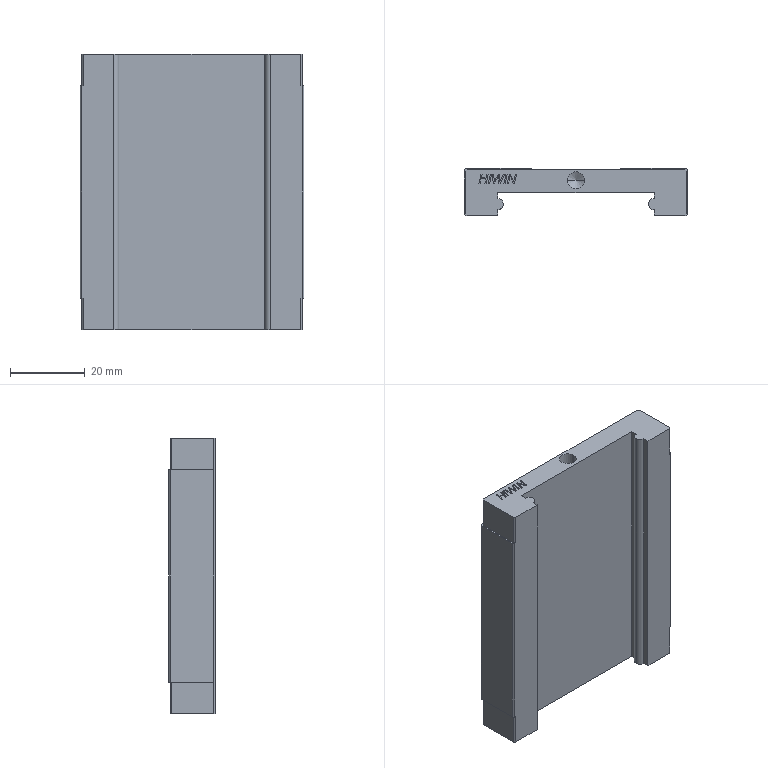Part | STEP file | Bag feed MGW15H slider | 1 solid | 210 faces | box 60 x 12.6 x 73.8 mm | volume 36057 mm3 | plane 137 | spline 44 | cylinder 17 | cone 12 | commonest cylinder face diameters 4 x8 4.5 x4 3 x3 0.6 x2